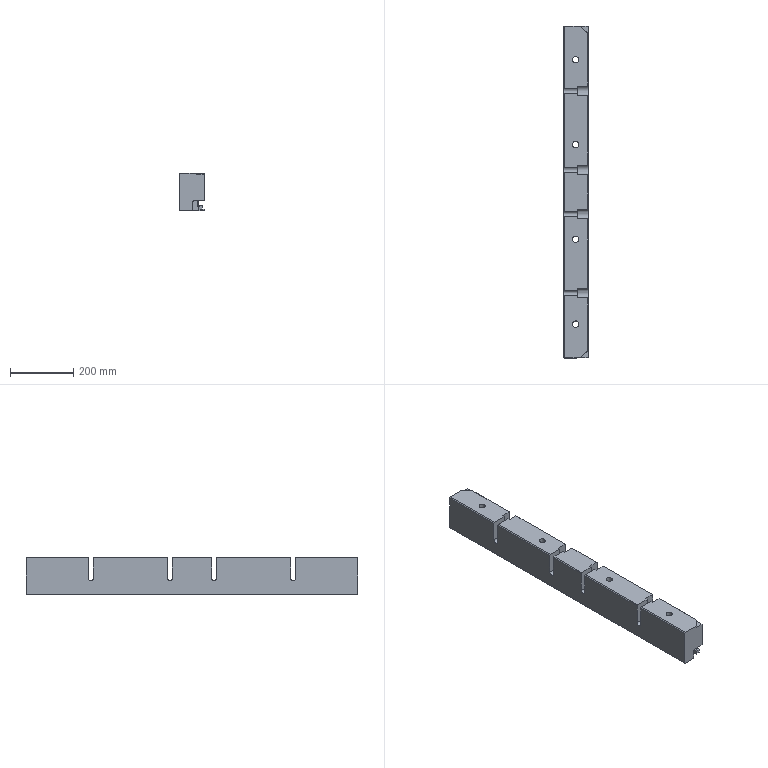Part | STEP file | 4-20.sldasm-Part-329 | 1 solid | 80 faces | box 78 x 1050 x 120 mm | volume 8694380 mm3 | plane 60 | cylinder 20 | commonest cylinder face diameters 19.842 x8 15.728 x4 30 x4 6 x3 14 x1